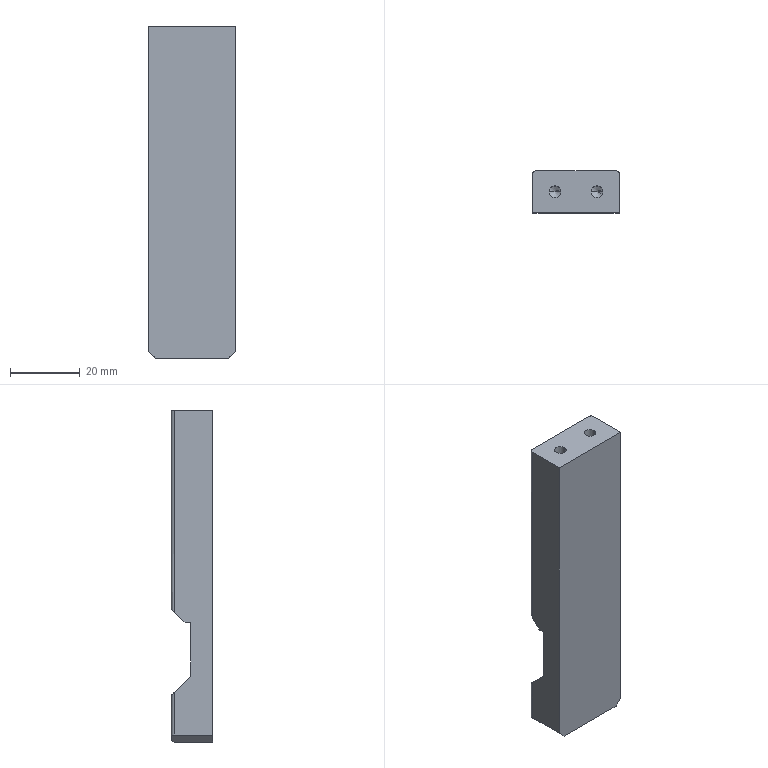Part | SolidWorks | features Chamfer 2, Cut 1, Extrusion 1, Fillet 1, HoleWzd 1, ICE 1 | 1 solid | 26 faces | box 25 x 12 x 95 mm | volume 25505 mm3 | plane 13 | cylinder 9 | cone 4 | commonest cylinder face diameters 2 x5 3.3 x4
STEP:
#1=CARTESIAN_POINT('',(4.85,0.,37.4));
#2=VERTEX_POINT('',#1);
#3=CARTESIAN_POINT('',(8.15,0.,37.4));
#4=VERTEX_POINT('',#3);
#5=CARTESIAN_POINT('',(6.5,0.,37.4));
#6=DIRECTION('',(0.,0.,1.));
#7=DIRECTION('',(1.,0.,0.));
#8=AXIS2_PLACEMENT_3D('',#5,#6,#7);
#9=CIRCLE('',#8,1.65);
#10=EDGE_CURVE('',#2,#4,#9,.T.);
#11=ORIENTED_EDGE('',*,*,#10,.F.);
#12=CARTESIAN_POINT('',(4.85,0.,47.5));
#13=VERTEX_POINT('',#12);
#14=CARTESIAN_POINT('',(4.85,0.,47.5));
#15=DIRECTION('',(0.,0.,1.));
#16=VECTOR('',#15,1000.);
#17=LINE('',#14,#16);
#18=EDGE_CURVE('',#2,#13,#17,.T.);
#19=ORIENTED_EDGE('',*,*,#18,.T.);
#20=CARTESIAN_POINT('',(8.15,0.,47.5));
#21=VERTEX_POINT('',#20);
#22=CARTESIAN_POINT('',(6.5,0.,47.5));
#23=DIRECTION('',(0.,0.,1.));
#24=DIRECTION('',(1.,0.,0.));
#25=AXIS2_PLACEMENT_3D('',#22,#23,#24);
#26=CIRCLE('',#25,1.65);
#27=EDGE_CURVE('',#13,#21,#26,.T.);
#28=ORIENTED_EDGE('',*,*,#27,.T.);
#29=CARTESIAN_POINT('',(8.15,0.,47.5));
#30=DIRECTION('',(0.,0.,1.));
#31=VECTOR('',#30,1000.);
#32=LINE('',#29,#31);
#33=EDGE_CURVE('',#4,#21,#32,.T.);
#34=ORIENTED_EDGE('',*,*,#33,.F.);
#35=EDGE_LOOP('',(#11,#19,#28,#34));
#36=FACE_OUTER_BOUND('',#35,.T.);
#37=CARTESIAN_POINT('',(6.5,0.,47.5));
#38=DIRECTION('',(0.,0.,1.));
#39=DIRECTION('',(1.,0.,0.));
#40=AXIS2_PLACEMENT_3D('',#37,#38,#39);
#41=CYLINDRICAL_SURFACE('',#40,1.65);
#42=ADVANCED_FACE('',(#36),#41,.F.);
#43=CARTESIAN_POINT('',(6.5,0.,36.409));
#44=VERTEX_POINT('',#43);
#45=CARTESIAN_POINT('',(8.15,0.,37.4));
#46=DIRECTION('',(0.8572,0.,0.515));
#47=VECTOR('',#46,1000.);
#48=LINE('',#45,#47);
#49=EDGE_CURVE('',#44,#4,#48,.T.);
#50=ORIENTED_EDGE('',*,*,#49,.F.);
#51=CARTESIAN_POINT('',(4.85,0.,37.4));
#52=DIRECTION('',(-0.8572,0.,0.515));
#53=VECTOR('',#52,1000.);
#54=LINE('',#51,#53);
#55=EDGE_CURVE('',#44,#2,#54,.T.);
#56=ORIENTED_EDGE('',*,*,#55,.T.);
#57=ORIENTED_EDGE('',*,*,#10,.T.);
#58=EDGE_LOOP('',(#50,#56,#57));
#59=FACE_OUTER_BOUND('',#58,.T.);
#60=CARTESIAN_POINT('',(6.5,0.,37.4));
#61=DIRECTION('',(0.,0.,1.));
#62=DIRECTION('',(1.,0.,0.));
#63=AXIS2_PLACEMENT_3D('',#60,#61,#62);
#64=CONICAL_SURFACE('',#63,1.65,1.03);
#65=ADVANCED_FACE('',(#59),#64,.F.);
#66=CARTESIAN_POINT('',(16.85,0.,37.4));
#67=VERTEX_POINT('',#66);
#68=CARTESIAN_POINT('',(20.15,0.,37.4));
#69=VERTEX_POINT('',#68);
#70=CARTESIAN_POINT('',(18.5,0.,37.4));
#71=DIRECTION('',(0.,0.,1.));
#72=DIRECTION('',(1.,0.,0.));
#73=AXIS2_PLACEMENT_3D('',#70,#71,#72);
#74=CIRCLE('',#73,1.65);
#75=EDGE_CURVE('',#67,#69,#74,.T.);
#76=ORIENTED_EDGE('',*,*,#75,.F.);
#77=CARTESIAN_POINT('',(16.85,0.,47.5));
#78=VERTEX_POINT('',#77);
#79=CARTESIAN_POINT('',(16.85,0.,47.5));
#80=DIRECTION('',(0.,0.,1.));
#81=VECTOR('',#80,1000.);
#82=LINE('',#79,#81);
#83=EDGE_CURVE('',#67,#78,#82,.T.);
#84=ORIENTED_EDGE('',*,*,#83,.T.);
#85=CARTESIAN_POINT('',(20.15,0.,47.5));
#86=VERTEX_POINT('',#85);
#87=CARTESIAN_POINT('',(18.5,0.,47.5));
#88=DIRECTION('',(0.,0.,1.));
#89=DIRECTION('',(1.,0.,0.));
#90=AXIS2_PLACEMENT_3D('',#87,#88,#89);
#91=CIRCLE('',#90,1.65);
#92=EDGE_CURVE('',#78,#86,#91,.T.);
#93=ORIENTED_EDGE('',*,*,#92,.T.);
#94=CARTESIAN_POINT('',(20.15,0.,47.5));
#95=DIRECTION('',(0.,0.,1.));
#96=VECTOR('',#95,1000.);
#97=LINE('',#94,#96);
#98=EDGE_CURVE('',#69,#86,#97,.T.);
#99=ORIENTED_EDGE('',*,*,#98,.F.);
#100=EDGE_LOOP('',(#76,#84,#93,#99));
#101=FACE_OUTER_BOUND('',#100,.T.);
#102=CARTESIAN_POINT('',(18.5,0.,47.5));
#103=DIRECTION('',(0.,0.,1.));
#104=DIRECTION('',(1.,0.,0.));
#105=AXIS2_PLACEMENT_3D('',#102,#103,#104);
#106=CYLINDRICAL_SURFACE('',#105,1.65);
#107=ADVANCED_FACE('',(#101),#106,.F.);
#108=CARTESIAN_POINT('',(18.5,0.,36.409));
#109=VERTEX_POINT('',#108);
#110=CARTESIAN_POINT('',(20.15,0.,37.4));
#111=DIRECTION('',(0.8572,0.,0.515));
#112=VECTOR('',#111,1000.);
#113=LINE('',#110,#112);
#114=EDGE_CURVE('',#109,#69,#113,.T.);
#115=ORIENTED_EDGE('',*,*,#114,.F.);
#116=CARTESIAN_POINT('',(16.85,0.,37.4));
#117=DIRECTION('',(-0.8572,0.,0.515));
#118=VECTOR('',#117,1000.);
#119=LINE('',#116,#118);
#120=EDGE_CURVE('',#109,#67,#119,.T.);
#121=ORIENTED_EDGE('',*,*,#120,.T.);
#122=ORIENTED_EDGE('',*,*,#75,.T.);
#123=EDGE_LOOP('',(#115,#121,#122));
#124=FACE_OUTER_BOUND('',#123,.T.);
#125=CARTESIAN_POINT('',(18.5,0.,37.4));
#126=DIRECTION('',(0.,0.,1.));
#127=DIRECTION('',(1.,0.,0.));
#128=AXIS2_PLACEMENT_3D('',#125,#126,#127);
#129=CONICAL_SURFACE('',#128,1.65,1.03);
#130=ADVANCED_FACE('',(#124),#129,.F.);
#131=CARTESIAN_POINT('',(1.,6.,-46.5));
#132=VERTEX_POINT('',#131);
#133=CARTESIAN_POINT('',(1.,6.,-34.25));
#134=VERTEX_POINT('',#133);
#135=CARTESIAN_POINT('',(1.,6.,-32.65));
#136=DIRECTION('',(0.,0.,1.));
#137=VECTOR('',#136,1000.);
#138=LINE('',#135,#137);
#139=EDGE_CURVE('',#132,#134,#138,.T.);
#140=ORIENTED_EDGE('',*,*,#139,.T.);
#141=CARTESIAN_POINT('',(24.,6.,-34.25));
#142=VERTEX_POINT('',#141);
#143=CARTESIAN_POINT('',(0.,6.,-34.25));
#144=DIRECTION('',(1.,0.,0.));
#145=VECTOR('',#144,1000.);
#146=LINE('',#143,#145);
#147=EDGE_CURVE('',#134,#142,#146,.T.);
#148=ORIENTED_EDGE('',*,*,#147,.T.);
#149=CARTESIAN_POINT('',(24.,6.,-46.5));
#150=VERTEX_POINT('',#149);
#151=CARTESIAN_POINT('',(24.,6.,47.5));
#152=DIRECTION('',(0.,0.,-1.));
#153=VECTOR('',#152,1000.);
#154=LINE('',#151,#153);
#155=EDGE_CURVE('',#142,#150,#154,.T.);
#156=ORIENTED_EDGE('',*,*,#155,.T.);
#157=CARTESIAN_POINT('',(25.,6.,-46.5));
#158=DIRECTION('',(-1.,0.,0.));
#159=VECTOR('',#158,1000.);
#160=LINE('',#157,#159);
#161=EDGE_CURVE('',#150,#132,#160,.T.);
#162=ORIENTED_EDGE('',*,*,#161,.T.);
#163=EDGE_LOOP('',(#140,#148,#156,#162));
#164=FACE_OUTER_BOUND('',#163,.T.);
#165=CARTESIAN_POINT('',(25.,6.,47.5));
#166=DIRECTION('',(0.,-1.,0.));
#167=DIRECTION('',(0.,0.,-1.));
#168=AXIS2_PLACEMENT_3D('',#165,#166,#167);
#169=PLANE('',#168);
#170=ADVANCED_FACE('',(#164),#169,.F.);
#171=CARTESIAN_POINT('',(2.,-6.,-47.5));
#172=VERTEX_POINT('',#171);
#173=CARTESIAN_POINT('',(2.,5.,-47.5));
#174=VERTEX_POINT('',#173);
#175=CARTESIAN_POINT('',(2.,6.,-47.5));
#176=DIRECTION('',(0.,1.,0.));
#177=VECTOR('',#176,1000.);
#178=LINE('',#175,#177);
#179=EDGE_CURVE('',#172,#174,#178,.T.);
#180=ORIENTED_EDGE('',*,*,#179,.T.);
#181=CARTESIAN_POINT('',(23.,5.,-47.5));
#182=VERTEX_POINT('',#181);
#183=CARTESIAN_POINT('',(25.,5.,-47.5));
#184=DIRECTION('',(1.,0.,0.));
#185=VECTOR('',#184,1000.);
#186=LINE('',#183,#185);
#187=EDGE_CURVE('',#174,#182,#186,.T.);
#188=ORIENTED_EDGE('',*,*,#187,.T.);
#189=CARTESIAN_POINT('',(23.,-6.,-47.5));
#190=VERTEX_POINT('',#189);
#191=CARTESIAN_POINT('',(23.,-6.,-47.5));
#192=DIRECTION('',(0.,-1.,0.));
#193=VECTOR('',#192,1000.);
#194=LINE('',#191,#193);
#195=EDGE_CURVE('',#182,#190,#194,.T.);
#196=ORIENTED_EDGE('',*,*,#195,.T.);
#197=CARTESIAN_POINT('',(25.,-6.,-47.5));
#198=DIRECTION('',(-1.,0.,0.));
#199=VECTOR('',#198,1000.);
#200=LINE('',#197,#199);
#201=EDGE_CURVE('',#190,#172,#200,.T.);
#202=ORIENTED_EDGE('',*,*,#201,.T.);
#203=EDGE_LOOP('',(#180,#188,#196,#202));
#204=FACE_OUTER_BOUND('',#203,.T.);
#205=CARTESIAN_POINT('',(25.,-6.,-47.5));
#206=DIRECTION('',(0.,0.,1.));
#207=DIRECTION('',(1.,0.,0.));
#208=AXIS2_PLACEMENT_3D('',#205,#206,#207);
#209=PLANE('',#208);
#210=ADVANCED_FACE('',(#204),#209,.F.);
#211=CARTESIAN_POINT('',(24.,6.,47.5));
#212=VERTEX_POINT('',#211);
#213=CARTESIAN_POINT('',(1.,6.,47.5));
#214=VERTEX_POINT('',#213);
#215=CARTESIAN_POINT('',(25.,6.,47.5));
#216=DIRECTION('',(-1.,0.,0.));
#217=VECTOR('',#216,1000.);
#218=LINE('',#215,#217);
#219=EDGE_CURVE('',#212,#214,#218,.T.);
#220=ORIENTED_EDGE('',*,*,#219,.F.);
#221=CARTESIAN_POINT('',(24.,6.,-9.35));
#222=VERTEX_POINT('',#221);
#223=CARTESIAN_POINT('',(24.,6.,47.5));
#224=DIRECTION('',(0.,0.,-1.));
#225=VECTOR('',#224,1000.);
#226=LINE('',#223,#225);
#227=EDGE_CURVE('',#212,#222,#226,.T.);
#228=ORIENTED_EDGE('',*,*,#227,.T.);
#229=CARTESIAN_POINT('',(1.,6.,-9.35));
#230=VERTEX_POINT('',#229);
#231=CARTESIAN_POINT('',(25.,6.,-9.35));
#232=DIRECTION('',(-1.,0.,0.));
#233=VECTOR('',#232,1000.);
#234=LINE('',#231,#233);
#235=EDGE_CURVE('',#222,#230,#234,.T.);
#236=ORIENTED_EDGE('',*,*,#235,.T.);
#237=CARTESIAN_POINT('',(1.,6.,47.5));
#238=DIRECTION('',(0.,0.,1.));
#239=VECTOR('',#238,1000.);
#240=LINE('',#237,#239);
#241=EDGE_CURVE('',#230,#214,#240,.T.);
#242=ORIENTED_EDGE('',*,*,#241,.T.);
#243=EDGE_LOOP('',(#220,#228,#236,#242));
#244=FACE_OUTER_BOUND('',#243,.T.);
#245=CARTESIAN_POINT('',(25.,6.,47.5));
#246=DIRECTION('',(0.,-1.,0.));
#247=DIRECTION('',(0.,0.,-1.));
#248=AXIS2_PLACEMENT_3D('',#245,#246,#247);
#249=PLANE('',#248);
#250=ADVANCED_FACE('',(#244),#249,.F.);
#251=CARTESIAN_POINT('',(6.5,0.,47.5));
#252=DIRECTION('',(0.,0.,1.));
#253=DIRECTION('',(1.,0.,0.));
#254=AXIS2_PLACEMENT_3D('',#251,#252,#253);
#255=CIRCLE('',#254,1.65);
#256=EDGE_CURVE('',#21,#13,#255,.T.);
#257=ORIENTED_EDGE('',*,*,#256,.F.);
#258=ORIENTED_EDGE('',*,*,#27,.F.);
#259=EDGE_LOOP('',(#257,#258));
#260=FACE_BOUND('',#259,.T.);
#261=CARTESIAN_POINT('',(18.5,0.,47.5));
#262=DIRECTION('',(0.,0.,1.));
#263=DIRECTION('',(1.,0.,0.));
#264=AXIS2_PLACEMENT_3D('',#261,#262,#263);
#265=CIRCLE('',#264,1.65);
#266=EDGE_CURVE('',#86,#78,#265,.T.);
#267=ORIENTED_EDGE('',*,*,#266,.F.);
#268=ORIENTED_EDGE('',*,*,#92,.F.);
#269=EDGE_LOOP('',(#267,#268));
#270=FACE_BOUND('',#269,.T.);
#271=CARTESIAN_POINT('',(25.,5.,47.5));
#272=VERTEX_POINT('',#271);
#273=CARTESIAN_POINT('',(25.,-6.,47.5));
#274=VERTEX_POINT('',#273);
#275=CARTESIAN_POINT('',(25.,-6.,47.5));
#276=DIRECTION('',(0.,-1.,0.));
#277=VECTOR('',#276,1000.);
#278=LINE('',#275,#277);
#279=EDGE_CURVE('',#272,#274,#278,.T.);
#280=ORIENTED_EDGE('',*,*,#279,.F.);
#281=CARTESIAN_POINT('',(24.,5.,47.5));
#282=DIRECTION('',(0.,0.,1.));
#283=DIRECTION('',(-1.,0.,0.));
#284=AXIS2_PLACEMENT_3D('',#281,#282,#283);
#285=CIRCLE('',#284,1.);
#286=EDGE_CURVE('',#272,#212,#285,.T.);
#287=ORIENTED_EDGE('',*,*,#286,.T.);
#288=ORIENTED_EDGE('',*,*,#219,.T.);
#289=CARTESIAN_POINT('',(0.,5.,47.5));
#290=VERTEX_POINT('',#289);
#291=CARTESIAN_POINT('',(1.,5.,47.5));
#292=DIRECTION('',(0.,0.,1.));
#293=DIRECTION('',(-1.,0.,0.));
#294=AXIS2_PLACEMENT_3D('',#291,#292,#293);
#295=CIRCLE('',#294,1.);
#296=EDGE_CURVE('',#214,#290,#295,.T.);
#297=ORIENTED_EDGE('',*,*,#296,.T.);
#298=CARTESIAN_POINT('',(0.,-6.,47.5));
#299=VERTEX_POINT('',#298);
#300=CARTESIAN_POINT('',(0.,-6.,47.5));
#301=DIRECTION('',(0.,-1.,0.));
#302=VECTOR('',#301,1000.);
#303=LINE('',#300,#302);
#304=EDGE_CURVE('',#290,#299,#303,.T.);
#305=ORIENTED_EDGE('',*,*,#304,.T.);
#306=CARTESIAN_POINT('',(25.,-6.,47.5));
#307=DIRECTION('',(-1.,0.,0.));
#308=VECTOR('',#307,1000.);
#309=LINE('',#306,#308);
#310=EDGE_CURVE('',#274,#299,#309,.T.);
#311=ORIENTED_EDGE('',*,*,#310,.F.);
#312=EDGE_LOOP('',(#280,#287,#288,#297,#305,#311));
#313=FACE_OUTER_BOUND('',#312,.T.);
#314=CARTESIAN_POINT('',(25.,-6.,47.5));
#315=DIRECTION('',(0.,0.,-1.));
#316=DIRECTION('',(-1.,0.,0.));
#317=AXIS2_PLACEMENT_3D('',#314,#315,#316);
#318=PLANE('',#317);
#319=ADVANCED_FACE('',(#260,#270,#313),#318,.F.);
#320=ORIENTED_EDGE('',*,*,#201,.F.);
#321=CARTESIAN_POINT('',(25.,-6.,-45.5));
#322=VERTEX_POINT('',#321);
#323=CARTESIAN_POINT('',(25.,-6.,-45.5));
#324=DIRECTION('',(0.7071,0.,0.7071));
#325=VECTOR('',#324,1000.);
#326=LINE('',#323,#325);
#327=EDGE_CURVE('',#190,#322,#326,.T.);
#328=ORIENTED_EDGE('',*,*,#327,.T.);
#329=CARTESIAN_POINT('',(25.,-6.,47.5));
#330=DIRECTION('',(0.,0.,-1.));
#331=VECTOR('',#330,1000.);
#332=LINE('',#329,#331);
#333=EDGE_CURVE('',#274,#322,#332,.T.);
#334=ORIENTED_EDGE('',*,*,#333,.F.);
#335=ORIENTED_EDGE('',*,*,#310,.T.);
#336=CARTESIAN_POINT('',(0.,-6.,-45.5));
#337=VERTEX_POINT('',#336);
#338=CARTESIAN_POINT('',(0.,-6.,47.5));
#339=DIRECTION('',(0.,0.,-1.));
#340=VECTOR('',#339,1000.);
#341=LINE('',#338,#340);
#342=EDGE_CURVE('',#299,#337,#341,.T.);
#343=ORIENTED_EDGE('',*,*,#342,.T.);
#344=CARTESIAN_POINT('',(2.,-6.,-47.5));
#345=DIRECTION('',(0.7071,0.,-0.7071));
#346=VECTOR('',#345,1000.);
#347=LINE('',#344,#346);
#348=EDGE_CURVE('',#337,#172,#347,.T.);
#349=ORIENTED_EDGE('',*,*,#348,.T.);
#350=EDGE_LOOP('',(#320,#328,#334,#335,#343,#349));
#351=FACE_OUTER_BOUND('',#350,.T.);
#352=CARTESIAN_POINT('',(25.,-6.,47.5));
#353=DIRECTION('',(0.,1.,0.));
#354=DIRECTION('',(0.,0.,1.));
#355=AXIS2_PLACEMENT_3D('',#352,#353,#354);
#356=PLANE('',#355);
#357=ADVANCED_FACE('',(#351),#356,.F.);
#358=CARTESIAN_POINT('',(25.,5.,-45.5));
#359=VERTEX_POINT('',#358);
#360=CARTESIAN_POINT('',(25.,5.,-33.25));
#361=VERTEX_POINT('',#360);
#362=CARTESIAN_POINT('',(25.,5.,0.));
#363=DIRECTION('',(0.,0.,1.));
#364=VECTOR('',#363,1000.);
#365=LINE('',#362,#364);
#366=EDGE_CURVE('',#359,#361,#365,.T.);
#367=ORIENTED_EDGE('',*,*,#366,.T.);
#368=CARTESIAN_POINT('',(25.,0.4,-28.65));
#369=VERTEX_POINT('',#368);
#370=CARTESIAN_POINT('',(25.,6.,-34.25));
#371=DIRECTION('',(0.,0.7071,-0.7071));
#372=VECTOR('',#371,1000.);
#373=LINE('',#370,#372);
#374=EDGE_CURVE('',#369,#361,#373,.T.);
#375=ORIENTED_EDGE('',*,*,#374,.F.);
#376=CARTESIAN_POINT('',(25.,0.4,-13.35));
#377=VERTEX_POINT('',#376);
#378=CARTESIAN_POINT('',(25.,0.4,-13.35));
#379=DIRECTION('',(0.,0.,-1.));
#380=VECTOR('',#379,1000.);
#381=LINE('',#378,#380);
#382=EDGE_CURVE('',#377,#369,#381,.T.);
#383=ORIENTED_EDGE('',*,*,#382,.F.);
#384=CARTESIAN_POINT('',(25.,2.,-13.35));
#385=VERTEX_POINT('',#384);
#386=CARTESIAN_POINT('',(25.,0.4,-13.35));
#387=DIRECTION('',(0.,1.,0.));
#388=VECTOR('',#387,1000.);
#389=LINE('',#386,#388);
#390=EDGE_CURVE('',#377,#385,#389,.T.);
#391=ORIENTED_EDGE('',*,*,#390,.T.);
#392=CARTESIAN_POINT('',(25.,5.,-10.35));
#393=VERTEX_POINT('',#392);
#394=CARTESIAN_POINT('',(25.,2.,-13.35));
#395=DIRECTION('',(0.,0.7071,0.7071));
#396=VECTOR('',#395,1000.);
#397=LINE('',#394,#396);
#398=EDGE_CURVE('',#385,#393,#397,.T.);
#399=ORIENTED_EDGE('',*,*,#398,.T.);
#400=CARTESIAN_POINT('',(25.,5.,0.));
#401=DIRECTION('',(0.,0.,1.));
#402=VECTOR('',#401,1000.);
#403=LINE('',#400,#402);
#404=EDGE_CURVE('',#393,#272,#403,.T.);
#405=ORIENTED_EDGE('',*,*,#404,.T.);
#406=ORIENTED_EDGE('',*,*,#279,.T.);
#407=ORIENTED_EDGE('',*,*,#333,.T.);
#408=CARTESIAN_POINT('',(25.,0.,-45.5));
#409=DIRECTION('',(0.,1.,0.));
#410=VECTOR('',#409,1000.);
#411=LINE('',#408,#410);
#412=EDGE_CURVE('',#322,#359,#411,.T.);
#413=ORIENTED_EDGE('',*,*,#412,.T.);
#414=EDGE_LOOP('',(#367,#375,#383,#391,#399,#405,#406,#407,#413));
#415=FACE_OUTER_BOUND('',#414,.T.);
#416=CARTESIAN_POINT('',(25.,0.,0.));
#417=DIRECTION('',(-1.,0.,0.));
#418=DIRECTION('',(0.,0.,1.));
#419=AXIS2_PLACEMENT_3D('',#416,#417,#418);
#420=PLANE('',#419);
#421=ADVANCED_FACE('',(#415),#420,.F.);
#422=CARTESIAN_POINT('',(0.,0.4,-28.65));
#423=VERTEX_POINT('',#422);
#424=CARTESIAN_POINT('',(0.,5.,-33.25));
#425=VERTEX_POINT('',#424);
#426=CARTESIAN_POINT('',(0.,6.,-34.25));
#427=DIRECTION('',(0.,0.7071,-0.7071));
#428=VECTOR('',#427,1000.);
#429=LINE('',#426,#428);
#430=EDGE_CURVE('',#423,#425,#429,.T.);
#431=ORIENTED_EDGE('',*,*,#430,.T.);
#432=CARTESIAN_POINT('',(0.,5.,-45.5));
#433=VERTEX_POINT('',#432);
#434=CARTESIAN_POINT('',(0.,5.,-45.5));
#435=DIRECTION('',(0.,0.,-1.));
#436=VECTOR('',#435,1000.);
#437=LINE('',#434,#436);
#438=EDGE_CURVE('',#425,#433,#437,.T.);
#439=ORIENTED_EDGE('',*,*,#438,.T.);
#440=CARTESIAN_POINT('',(0.,-6.,-45.5));
#441=DIRECTION('',(0.,-1.,0.));
#442=VECTOR('',#441,1000.);
#443=LINE('',#440,#442);
#444=EDGE_CURVE('',#433,#337,#443,.T.);
#445=ORIENTED_EDGE('',*,*,#444,.T.);
#446=ORIENTED_EDGE('',*,*,#342,.F.);
#447=ORIENTED_EDGE('',*,*,#304,.F.);
#448=CARTESIAN_POINT('',(0.,5.,-10.35));
#449=VERTEX_POINT('',#448);
#450=CARTESIAN_POINT('',(0.,5.,-9.35));
#451=DIRECTION('',(0.,0.,-1.));
#452=VECTOR('',#451,1000.);
#453=LINE('',#450,#452);
#454=EDGE_CURVE('',#290,#449,#453,.T.);
#455=ORIENTED_EDGE('',*,*,#454,.T.);
#456=CARTESIAN_POINT('',(0.,2.,-13.35));
#457=VERTEX_POINT('',#456);
#458=CARTESIAN_POINT('',(0.,7.675,-7.675));
#459=DIRECTION('',(0.,-0.7071,-0.7071));
#460=VECTOR('',#459,1000.);
#461=LINE('',#458,#460);
#462=EDGE_CURVE('',#449,#457,#461,.T.);
#463=ORIENTED_EDGE('',*,*,#462,.T.);
#464=CARTESIAN_POINT('',(0.,0.4,-13.35));
#465=VERTEX_POINT('',#464);
#466=CARTESIAN_POINT('',(0.,0.4,-13.35));
#467=DIRECTION('',(0.,1.,0.));
#468=VECTOR('',#467,1000.);
#469=LINE('',#466,#468);
#470=EDGE_CURVE('',#465,#457,#469,.T.);
#471=ORIENTED_EDGE('',*,*,#470,.F.);
#472=CARTESIAN_POINT('',(0.,0.4,-13.35));
#473=DIRECTION('',(0.,0.,1.));
#474=VECTOR('',#473,1000.);
#475=LINE('',#472,#474);
#476=EDGE_CURVE('',#423,#465,#475,.T.);
#477=ORIENTED_EDGE('',*,*,#476,.F.);
#478=EDGE_LOOP('',(#431,#439,#445,#446,#447,#455,#463,#471,#477));
#479=FACE_OUTER_BOUND('',#478,.T.);
#480=CARTESIAN_POINT('',(0.,0.,0.));
#481=DIRECTION('',(-1.,0.,0.));
#482=DIRECTION('',(0.,0.,1.));
#483=AXIS2_PLACEMENT_3D('',#480,#481,#482);
#484=PLANE('',#483);
#485=ADVANCED_FACE('',(#479),#484,.T.);
#486=ORIENTED_EDGE('',*,*,#470,.T.);
#487=CARTESIAN_POINT('',(25.,2.,-13.35));
#488=DIRECTION('',(1.,0.,0.));
#489=VECTOR('',#488,1000.);
#490=LINE('',#487,#489);
#491=EDGE_CURVE('',#457,#385,#490,.T.);
#492=ORIENTED_EDGE('',*,*,#491,.T.);
#493=ORIENTED_EDGE('',*,*,#390,.F.);
#494=CARTESIAN_POINT('',(25.,0.4,-13.35));
#495=DIRECTION('',(1.,0.,0.));
#496=VECTOR('',#495,1000.);
#497=LINE('',#494,#496);
#498=EDGE_CURVE('',#465,#377,#497,.T.);
#499=ORIENTED_EDGE('',*,*,#498,.F.);
#500=EDGE_LOOP('',(#486,#492,#493,#499));
#501=FACE_OUTER_BOUND('',#500,.T.);
#502=CARTESIAN_POINT('',(25.,0.4,-13.35));
#503=DIRECTION('',(0.,0.,1.));
#504=DIRECTION('',(1.,0.,0.));
#505=AXIS2_PLACEMENT_3D('',#502,#503,#504);
#506=PLANE('',#505);
#507=ADVANCED_FACE('',(#501),#506,.F.);
#508=ORIENTED_EDGE('',*,*,#476,.T.);
#509=ORIENTED_EDGE('',*,*,#498,.T.);
#510=ORIENTED_EDGE('',*,*,#382,.T.);
#511=CARTESIAN_POINT('',(25.,0.4,-28.65));
#512=DIRECTION('',(-1.,0.,0.));
#513=VECTOR('',#512,1000.);
#514=LINE('',#511,#513);
#515=EDGE_CURVE('',#369,#423,#514,.T.);
#516=ORIENTED_EDGE('',*,*,#515,.T.);
#517=EDGE_LOOP('',(#508,#509,#510,#516));
#518=FACE_OUTER_BOUND('',#517,.T.);
#519=CARTESIAN_POINT('',(0.,0.4,0.));
#520=DIRECTION('',(0.,1.,0.));
#521=DIRECTION('',(0.,0.,1.));
#522=AXIS2_PLACEMENT_3D('',#519,#520,#521);
#523=PLANE('',#522);
#524=ADVANCED_FACE('',(#518),#523,.T.);
#525=ORIENTED_EDGE('',*,*,#235,.F.);
#526=CARTESIAN_POINT('',(24.,6.,-9.35));
#527=CARTESIAN_POINT('',(24.586,6.,-9.35));
#528=CARTESIAN_POINT('',(25.,5.586,-9.764));
#529=CARTESIAN_POINT('',(25.,5.,-10.35));
#530=(BOUNDED_CURVE()B_SPLINE_CURVE(3,(#526,#527,#528,#529),.UNSPECIFIED.,.F.,.F.)B_SPLINE_CURVE_WITH_KNOTS((4,4),(0.,1.571),.UNSPECIFIED.)CURVE()GEOMETRIC_REPRESENTATION_ITEM()RATIONAL_B_SPLINE_CURVE((1.,0.8047,0.8047,1.))REPRESENTATION_ITEM(''));
#531=EDGE_CURVE('',#222,#393,#530,.T.);
#532=ORIENTED_EDGE('',*,*,#531,.T.);
#533=ORIENTED_EDGE('',*,*,#398,.F.);
#534=ORIENTED_EDGE('',*,*,#491,.F.);
#535=ORIENTED_EDGE('',*,*,#462,.F.);
#536=CARTESIAN_POINT('',(0.,5.,-10.35));
#537=CARTESIAN_POINT('',(0.,5.586,-9.764));
#538=CARTESIAN_POINT('',(0.4142,6.,-9.35));
#539=CARTESIAN_POINT('',(1.,6.,-9.35));
#540=(BOUNDED_CURVE()B_SPLINE_CURVE(3,(#536,#537,#538,#539),.UNSPECIFIED.,.F.,.F.)B_SPLINE_CURVE_WITH_KNOTS((4,4),(1.571,3.142),.UNSPECIFIED.)CURVE()GEOMETRIC_REPRESENTATION_ITEM()RATIONAL_B_SPLINE_CURVE((1.,0.8047,0.8047,1.))REPRESENTATION_ITEM(''));
#541=EDGE_CURVE('',#449,#230,#540,.T.);
#542=ORIENTED_EDGE('',*,*,#541,.T.);
#543=EDGE_LOOP('',(#525,#532,#533,#534,#535,#542));
#544=FACE_OUTER_BOUND('',#543,.T.);
#545=CARTESIAN_POINT('',(25.,2.,-13.35));
#546=DIRECTION('',(0.,-0.7071,0.7071));
#547=DIRECTION('',(1.,0.,0.));
#548=AXIS2_PLACEMENT_3D('',#545,#546,#547);
#549=PLANE('',#548);
#550=ADVANCED_FACE('',(#544),#549,.F.);
#551=ORIENTED_EDGE('',*,*,#195,.F.);
#552=CARTESIAN_POINT('',(23.,5.,-47.5));
#553=CARTESIAN_POINT('',(23.,5.586,-47.5));
#554=CARTESIAN_POINT('',(23.414,6.,-47.086));
#555=CARTESIAN_POINT('',(24.,6.,-46.5));
#556=(BOUNDED_CURVE()B_SPLINE_CURVE(3,(#552,#553,#554,#555),.UNSPECIFIED.,.F.,.F.)B_SPLINE_CURVE_WITH_KNOTS((4,4),(0.,1.571),.UNSPECIFIED.)CURVE()GEOMETRIC_REPRESENTATION_ITEM()RATIONAL_B_SPLINE_CURVE((1.,0.8047,0.8047,1.))REPRESENTATION_ITEM(''));
#557=EDGE_CURVE('',#182,#150,#556,.T.);
#558=ORIENTED_EDGE('',*,*,#557,.T.);
#559=CARTESIAN_POINT('',(24.,6.,-46.5));
#560=CARTESIAN_POINT('',(24.586,6.,-45.914));
#561=CARTESIAN_POINT('',(25.,5.586,-45.5));
#562=CARTESIAN_POINT('',(25.,5.,-45.5));
#563=(BOUNDED_CURVE()B_SPLINE_CURVE(3,(#559,#560,#561,#562),.UNSPECIFIED.,.F.,.F.)B_SPLINE_CURVE_WITH_KNOTS((4,4),(4.712,6.283),.UNSPECIFIED.)CURVE()GEOMETRIC_REPRESENTATION_ITEM()RATIONAL_B_SPLINE_CURVE((1.,0.8047,0.8047,1.))REPRESENTATION_ITEM(''));
#564=EDGE_CURVE('',#150,#359,#563,.T.);
#565=ORIENTED_EDGE('',*,*,#564,.T.);
#566=ORIENTED_EDGE('',*,*,#412,.F.);
#567=ORIENTED_EDGE('',*,*,#327,.F.);
#568=EDGE_LOOP('',(#551,#558,#565,#566,#567));
#569=FACE_OUTER_BOUND('',#568,.T.);
#570=CARTESIAN_POINT('',(25.,0.,-45.5));
#571=DIRECTION('',(-0.7071,0.,0.7071));
#572=DIRECTION('',(0.,1.,0.));
#573=AXIS2_PLACEMENT_3D('',#570,#571,#572);
#574=PLANE('',#573);
#575=ADVANCED_FACE('',(#569),#574,.F.);
#576=CARTESIAN_POINT('',(0.,5.,-45.5));
#577=CARTESIAN_POINT('',(0.,5.586,-45.5));
#578=CARTESIAN_POINT('',(0.4142,6.,-45.914));
#579=CARTESIAN_POINT('',(1.,6.,-46.5));
#580=(BOUNDED_CURVE()B_SPLINE_CURVE(3,(#576,#577,#578,#579),.UNSPECIFIED.,.F.,.F.)B_SPLINE_CURVE_WITH_KNOTS((4,4),(3.142,4.712),.UNSPECIFIED.)CURVE()GEOMETRIC_REPRESENTATION_ITEM()RATIONAL_B_SPLINE_CURVE((1.,0.8047,0.8047,1.))REPRESENTATION_ITEM(''));
#581=EDGE_CURVE('',#433,#132,#580,.T.);
#582=ORIENTED_EDGE('',*,*,#581,.T.);
#583=CARTESIAN_POINT('',(1.,6.,-46.5));
#584=CARTESIAN_POINT('',(1.586,6.,-47.086));
#585=CARTESIAN_POINT('',(2.,5.586,-47.5));
#586=CARTESIAN_POINT('',(2.,5.,-47.5));
#587=(BOUNDED_CURVE()B_SPLINE_CURVE(3,(#583,#584,#585,#586),.UNSPECIFIED.,.F.,.F.)B_SPLINE_CURVE_WITH_KNOTS((4,4),(1.571,3.142),.UNSPECIFIED.)CURVE()GEOMETRIC_REPRESENTATION_ITEM()RATIONAL_B_SPLINE_CURVE((1.,0.8047,0.8047,1.))REPRESENTATION_ITEM(''));
#588=EDGE_CURVE('',#132,#174,#587,.T.);
#589=ORIENTED_EDGE('',*,*,#588,.T.);
#590=ORIENTED_EDGE('',*,*,#179,.F.);
#591=ORIENTED_EDGE('',*,*,#348,.F.);
#592=ORIENTED_EDGE('',*,*,#444,.F.);
#593=EDGE_LOOP('',(#582,#589,#590,#591,#592));
#594=FACE_OUTER_BOUND('',#593,.T.);
#595=CARTESIAN_POINT('',(2.,-6.,-47.5));
#596=DIRECTION('',(-0.7071,0.,-0.7071));
#597=DIRECTION('',(0.,-1.,0.));
#598=AXIS2_PLACEMENT_3D('',#595,#596,#597);
#599=PLANE('',#598);
#600=ADVANCED_FACE('',(#594),#599,.T.);
#601=ORIENTED_EDGE('',*,*,#120,.F.);
#602=ORIENTED_EDGE('',*,*,#114,.T.);
#603=CARTESIAN_POINT('',(18.5,0.,37.4));
#604=DIRECTION('',(0.,0.,1.));
#605=DIRECTION('',(1.,0.,0.));
#606=AXIS2_PLACEMENT_3D('',#603,#604,#605);
#607=CIRCLE('',#606,1.65);
#608=EDGE_CURVE('',#69,#67,#607,.T.);
#609=ORIENTED_EDGE('',*,*,#608,.T.);
#610=EDGE_LOOP('',(#601,#602,#609));
#611=FACE_OUTER_BOUND('',#610,.T.);
#612=CARTESIAN_POINT('',(18.5,0.,37.4));
#613=DIRECTION('',(0.,0.,1.));
#614=DIRECTION('',(1.,0.,0.));
#615=AXIS2_PLACEMENT_3D('',#612,#613,#614);
#616=CONICAL_SURFACE('',#615,1.65,1.03);
#617=ADVANCED_FACE('',(#611),#616,.F.);
#618=ORIENTED_EDGE('',*,*,#83,.F.);
#619=ORIENTED_EDGE('',*,*,#608,.F.);
#620=ORIENTED_EDGE('',*,*,#98,.T.);
#621=ORIENTED_EDGE('',*,*,#266,.T.);
#622=EDGE_LOOP('',(#618,#619,#620,#621));
#623=FACE_OUTER_BOUND('',#622,.T.);
#624=CARTESIAN_POINT('',(18.5,0.,47.5));
#625=DIRECTION('',(0.,0.,1.));
#626=DIRECTION('',(1.,0.,0.));
#627=AXIS2_PLACEMENT_3D('',#624,#625,#626);
#628=CYLINDRICAL_SURFACE('',#627,1.65);
#629=ADVANCED_FACE('',(#623),#628,.F.);
#630=ORIENTED_EDGE('',*,*,#55,.F.);
#631=ORIENTED_EDGE('',*,*,#49,.T.);
#632=CARTESIAN_POINT('',(6.5,0.,37.4));
#633=DIRECTION('',(0.,0.,1.));
#634=DIRECTION('',(1.,0.,0.));
#635=AXIS2_PLACEMENT_3D('',#632,#633,#634);
#636=CIRCLE('',#635,1.65);
#637=EDGE_CURVE('',#4,#2,#636,.T.);
#638=ORIENTED_EDGE('',*,*,#637,.T.);
#639=EDGE_LOOP('',(#630,#631,#638));
#640=FACE_OUTER_BOUND('',#639,.T.);
#641=CARTESIAN_POINT('',(6.5,0.,37.4));
#642=DIRECTION('',(0.,0.,1.));
#643=DIRECTION('',(1.,0.,0.));
#644=AXIS2_PLACEMENT_3D('',#641,#642,#643);
#645=CONICAL_SURFACE('',#644,1.65,1.03);
#646=ADVANCED_FACE('',(#640),#645,.F.);
#647=ORIENTED_EDGE('',*,*,#18,.F.);
#648=ORIENTED_EDGE('',*,*,#637,.F.);
#649=ORIENTED_EDGE('',*,*,#33,.T.);
#650=ORIENTED_EDGE('',*,*,#256,.T.);
#651=EDGE_LOOP('',(#647,#648,#649,#650));
#652=FACE_OUTER_BOUND('',#651,.T.);
#653=CARTESIAN_POINT('',(6.5,0.,47.5));
#654=DIRECTION('',(0.,0.,1.));
#655=DIRECTION('',(1.,0.,0.));
#656=AXIS2_PLACEMENT_3D('',#653,#654,#655);
#657=CYLINDRICAL_SURFACE('',#656,1.65);
#658=ADVANCED_FACE('',(#652),#657,.F.);
#659=ORIENTED_EDGE('',*,*,#557,.F.);
#660=ORIENTED_EDGE('',*,*,#187,.F.);
#661=ORIENTED_EDGE('',*,*,#588,.F.);
#662=ORIENTED_EDGE('',*,*,#161,.F.);
#663=EDGE_LOOP('',(#659,#660,#661,#662));
#664=FACE_OUTER_BOUND('',#663,.T.);
#665=CARTESIAN_POINT('',(25.,5.,-46.5));
#666=DIRECTION('',(-1.,0.,0.));
#667=DIRECTION('',(0.,0.,1.));
#668=AXIS2_PLACEMENT_3D('',#665,#666,#667);
#669=CYLINDRICAL_SURFACE('',#668,1.);
#670=ADVANCED_FACE('',(#664),#669,.T.);
#671=ORIENTED_EDGE('',*,*,#531,.F.);
#672=ORIENTED_EDGE('',*,*,#227,.F.);
#673=ORIENTED_EDGE('',*,*,#286,.F.);
#674=ORIENTED_EDGE('',*,*,#404,.F.);
#675=EDGE_LOOP('',(#671,#672,#673,#674));
#676=FACE_OUTER_BOUND('',#675,.T.);
#677=CARTESIAN_POINT('',(24.,5.,0.));
#678=DIRECTION('',(0.,0.,1.));
#679=DIRECTION('',(1.,0.,0.));
#680=AXIS2_PLACEMENT_3D('',#677,#678,#679);
#681=CYLINDRICAL_SURFACE('',#680,1.);
#682=ADVANCED_FACE('',(#676),#681,.T.);
#683=CARTESIAN_POINT('',(25.,5.,-33.25));
#684=CARTESIAN_POINT('',(25.,5.586,-33.836));
#685=CARTESIAN_POINT('',(24.586,6.,-34.25));
#686=CARTESIAN_POINT('',(24.,6.,-34.25));
#687=(BOUNDED_CURVE()B_SPLINE_CURVE(3,(#683,#684,#685,#686),.UNSPECIFIED.,.F.,.F.)B_SPLINE_CURVE_WITH_KNOTS((4,4),(1.571,3.142),.UNSPECIFIED.)CURVE()GEOMETRIC_REPRESENTATION_ITEM()RATIONAL_B_SPLINE_CURVE((1.,0.8047,0.8047,1.))REPRESENTATION_ITEM(''));
#688=EDGE_CURVE('',#361,#142,#687,.T.);
#689=ORIENTED_EDGE('',*,*,#688,.F.);
#690=ORIENTED_EDGE('',*,*,#366,.F.);
#691=ORIENTED_EDGE('',*,*,#564,.F.);
#692=ORIENTED_EDGE('',*,*,#155,.F.);
#693=EDGE_LOOP('',(#689,#690,#691,#692));
#694=FACE_OUTER_BOUND('',#693,.T.);
#695=CARTESIAN_POINT('',(24.,5.,0.));
#696=DIRECTION('',(0.,0.,1.));
#697=DIRECTION('',(1.,0.,0.));
#698=AXIS2_PLACEMENT_3D('',#695,#696,#697);
#699=CYLINDRICAL_SURFACE('',#698,1.);
#700=ADVANCED_FACE('',(#694),#699,.T.);
#701=CARTESIAN_POINT('',(1.,6.,-34.25));
#702=CARTESIAN_POINT('',(0.4142,6.,-34.25));
#703=CARTESIAN_POINT('',(0.,5.586,-33.836));
#704=CARTESIAN_POINT('',(0.,5.,-33.25));
#705=(BOUNDED_CURVE()B_SPLINE_CURVE(3,(#701,#702,#703,#704),.UNSPECIFIED.,.F.,.F.)B_SPLINE_CURVE_WITH_KNOTS((4,4),(0.,1.571),.UNSPECIFIED.)CURVE()GEOMETRIC_REPRESENTATION_ITEM()RATIONAL_B_SPLINE_CURVE((1.,0.8047,0.8047,1.))REPRESENTATION_ITEM(''));
#706=EDGE_CURVE('',#134,#425,#705,.T.);
#707=ORIENTED_EDGE('',*,*,#706,.F.);
#708=ORIENTED_EDGE('',*,*,#139,.F.);
#709=ORIENTED_EDGE('',*,*,#581,.F.);
#710=ORIENTED_EDGE('',*,*,#438,.F.);
#711=EDGE_LOOP('',(#707,#708,#709,#710));
#712=FACE_OUTER_BOUND('',#711,.T.);
#713=CARTESIAN_POINT('',(1.,5.,47.5));
#714=DIRECTION('',(0.,0.,-1.));
#715=DIRECTION('',(-1.,0.,0.));
#716=AXIS2_PLACEMENT_3D('',#713,#714,#715);
#717=CYLINDRICAL_SURFACE('',#716,1.);
#718=ADVANCED_FACE('',(#712),#717,.T.);
#719=ORIENTED_EDGE('',*,*,#541,.F.);
#720=ORIENTED_EDGE('',*,*,#454,.F.);
#721=ORIENTED_EDGE('',*,*,#296,.F.);
#722=ORIENTED_EDGE('',*,*,#241,.F.);
#723=EDGE_LOOP('',(#719,#720,#721,#722));
#724=FACE_OUTER_BOUND('',#723,.T.);
#725=CARTESIAN_POINT('',(1.,5.,47.5));
#726=DIRECTION('',(0.,0.,-1.));
#727=DIRECTION('',(-1.,0.,0.));
#728=AXIS2_PLACEMENT_3D('',#725,#726,#727);
#729=CYLINDRICAL_SURFACE('',#728,1.);
#730=ADVANCED_FACE('',(#724),#729,.T.);
#731=ORIENTED_EDGE('',*,*,#688,.T.);
#732=ORIENTED_EDGE('',*,*,#147,.F.);
#733=ORIENTED_EDGE('',*,*,#706,.T.);
#734=ORIENTED_EDGE('',*,*,#430,.F.);
#735=ORIENTED_EDGE('',*,*,#515,.F.);
#736=ORIENTED_EDGE('',*,*,#374,.T.);
#737=EDGE_LOOP('',(#731,#732,#733,#734,#735,#736));
#738=FACE_OUTER_BOUND('',#737,.T.);
#739=CARTESIAN_POINT('',(0.,6.,-34.25));
#740=DIRECTION('',(0.,-0.7071,-0.7071));
#741=DIRECTION('',(0.,0.7071,-0.7071));
#742=AXIS2_PLACEMENT_3D('',#739,#740,#741);
#743=PLANE('',#742);
#744=ADVANCED_FACE('',(#738),#743,.F.);
#745=CLOSED_SHELL('',(#42,#65,#107,#130,#170,#210,#250,#319,#357,#421,#485,#507,#524,#550,#575,#600,#617,#629,#646,#658,#670,#682,#700,#718,#730,#744));
#746=MANIFOLD_SOLID_BREP('',#745);
#747=CARTESIAN_POINT('',(0.,0.,0.));
#748=DIRECTION('',(0.,0.,1.));
#749=DIRECTION('',(1.,0.,0.));
#750=AXIS2_PLACEMENT_3D('',#747,#748,#749);
#751=(LENGTH_UNIT()NAMED_UNIT(*)SI_UNIT(.MILLI.,.METRE.));
#752=UNCERTAINTY_MEASURE_WITH_UNIT(LENGTH_MEASURE(0.00001),#751,'','');
#753=(NAMED_UNIT(*)PLANE_ANGLE_UNIT()SI_UNIT($,.RADIAN.));
#754=(NAMED_UNIT(*)SI_UNIT($,.STERADIAN.)SOLID_ANGLE_UNIT());
#755=(GEOMETRIC_REPRESENTATION_CONTEXT(3)GLOBAL_UNCERTAINTY_ASSIGNED_CONTEXT((#752))GLOBAL_UNIT_ASSIGNED_CONTEXT((#751,#753,#754))REPRESENTATION_CONTEXT('',''));
#756=ADVANCED_BREP_SHAPE_REPRESENTATION('',(#746,#750),#755);